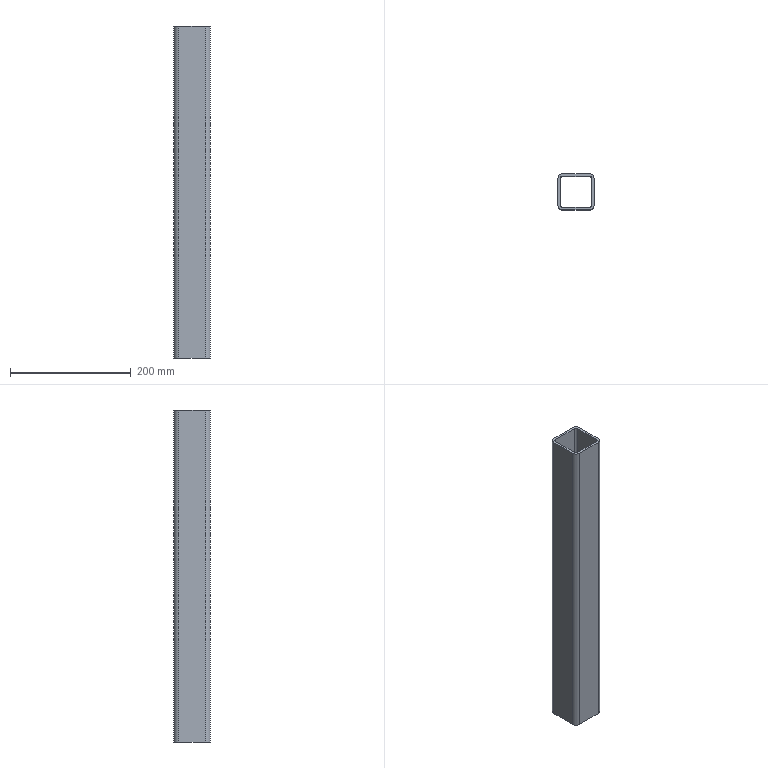Part | SolidWorks | features BaseBody 1 | 1 solid | 18 faces | box 60 x 60 x 550 mm | volume 470138 mm3 | plane 10 | cylinder 8 | commonest cylinder face diameters 8 x4 16 x4
STEP:
#1=CARTESIAN_POINT('',(644.,44.,-1270.));
#2=VERTEX_POINT('',#1);
#3=CARTESIAN_POINT('',(644.,44.,-720.));
#4=VERTEX_POINT('',#3);
#5=CARTESIAN_POINT('',(644.,44.,530.));
#6=DIRECTION('',(0.,0.,1.));
#7=VECTOR('',#6,1000.);
#8=LINE('',#5,#7);
#9=EDGE_CURVE('',#2,#4,#8,.T.);
#10=ORIENTED_EDGE('',*,*,#9,.T.);
#11=CARTESIAN_POINT('',(644.,0.,-720.));
#12=VERTEX_POINT('',#11);
#13=CARTESIAN_POINT('',(644.,44.,-720.));
#14=DIRECTION('',(0.,-1.,0.));
#15=VECTOR('',#14,1000.);
#16=LINE('',#13,#15);
#17=EDGE_CURVE('',#4,#12,#16,.T.);
#18=ORIENTED_EDGE('',*,*,#17,.T.);
#19=CARTESIAN_POINT('',(644.,0.,-1270.));
#20=VERTEX_POINT('',#19);
#21=CARTESIAN_POINT('',(644.,0.,530.));
#22=DIRECTION('',(0.,0.,-1.));
#23=VECTOR('',#22,1000.);
#24=LINE('',#21,#23);
#25=EDGE_CURVE('',#12,#20,#24,.T.);
#26=ORIENTED_EDGE('',*,*,#25,.T.);
#27=CARTESIAN_POINT('',(644.,44.,-1270.));
#28=DIRECTION('',(0.,1.,0.));
#29=VECTOR('',#28,1000.);
#30=LINE('',#27,#29);
#31=EDGE_CURVE('',#20,#2,#30,.T.);
#32=ORIENTED_EDGE('',*,*,#31,.T.);
#33=EDGE_LOOP('',(#10,#18,#26,#32));
#34=FACE_OUTER_BOUND('',#33,.T.);
#35=CARTESIAN_POINT('',(644.,44.,530.));
#36=DIRECTION('',(1.,0.,0.));
#37=DIRECTION('',(0.,0.,-1.));
#38=AXIS2_PLACEMENT_3D('',#35,#36,#37);
#39=PLANE('',#38);
#40=ADVANCED_FACE('',(#34),#39,.T.);
#41=ORIENTED_EDGE('',*,*,#17,.F.);
#42=CARTESIAN_POINT('',(648.,48.,-720.));
#43=VERTEX_POINT('',#42);
#44=CARTESIAN_POINT('',(648.,44.,-720.));
#45=DIRECTION('',(0.,0.,1.));
#46=DIRECTION('',(-1.,0.,0.));
#47=AXIS2_PLACEMENT_3D('',#44,#45,#46);
#48=CIRCLE('',#47,4.);
#49=EDGE_CURVE('',#43,#4,#48,.T.);
#50=ORIENTED_EDGE('',*,*,#49,.F.);
#51=CARTESIAN_POINT('',(692.,48.,-720.));
#52=VERTEX_POINT('',#51);
#53=CARTESIAN_POINT('',(0.,48.,-720.));
#54=DIRECTION('',(-1.,0.,0.));
#55=VECTOR('',#54,1000.);
#56=LINE('',#53,#55);
#57=EDGE_CURVE('',#52,#43,#56,.T.);
#58=ORIENTED_EDGE('',*,*,#57,.F.);
#59=CARTESIAN_POINT('',(696.,44.,-720.));
#60=VERTEX_POINT('',#59);
#61=CARTESIAN_POINT('',(692.,44.,-720.));
#62=DIRECTION('',(0.,0.,1.));
#63=DIRECTION('',(-1.,0.,0.));
#64=AXIS2_PLACEMENT_3D('',#61,#62,#63);
#65=CIRCLE('',#64,4.);
#66=EDGE_CURVE('',#60,#52,#65,.T.);
#67=ORIENTED_EDGE('',*,*,#66,.F.);
#68=CARTESIAN_POINT('',(696.,0.,-720.));
#69=VERTEX_POINT('',#68);
#70=CARTESIAN_POINT('',(696.,1242.,-720.));
#71=DIRECTION('',(0.,1.,0.));
#72=VECTOR('',#71,1000.);
#73=LINE('',#70,#72);
#74=EDGE_CURVE('',#69,#60,#73,.T.);
#75=ORIENTED_EDGE('',*,*,#74,.F.);
#76=CARTESIAN_POINT('',(692.,-4.,-720.));
#77=VERTEX_POINT('',#76);
#78=CARTESIAN_POINT('',(692.,0.,-720.));
#79=DIRECTION('',(0.,0.,1.));
#80=DIRECTION('',(-1.,0.,0.));
#81=AXIS2_PLACEMENT_3D('',#78,#79,#80);
#82=CIRCLE('',#81,4.);
#83=EDGE_CURVE('',#77,#69,#82,.T.);
#84=ORIENTED_EDGE('',*,*,#83,.F.);
#85=CARTESIAN_POINT('',(648.,-4.,-720.));
#86=VERTEX_POINT('',#85);
#87=CARTESIAN_POINT('',(0.,-4.,-720.));
#88=DIRECTION('',(1.,0.,0.));
#89=VECTOR('',#88,1000.);
#90=LINE('',#87,#89);
#91=EDGE_CURVE('',#86,#77,#90,.T.);
#92=ORIENTED_EDGE('',*,*,#91,.F.);
#93=CARTESIAN_POINT('',(648.,0.,-720.));
#94=DIRECTION('',(0.,0.,1.));
#95=DIRECTION('',(-1.,0.,0.));
#96=AXIS2_PLACEMENT_3D('',#93,#94,#95);
#97=CIRCLE('',#96,4.);
#98=EDGE_CURVE('',#12,#86,#97,.T.);
#99=ORIENTED_EDGE('',*,*,#98,.F.);
#100=EDGE_LOOP('',(#41,#50,#58,#67,#75,#84,#92,#99));
#101=FACE_BOUND('',#100,.T.);
#102=CARTESIAN_POINT('',(648.,-8.,-720.));
#103=VERTEX_POINT('',#102);
#104=CARTESIAN_POINT('',(640.,0.,-720.));
#105=VERTEX_POINT('',#104);
#106=CARTESIAN_POINT('',(648.,0.,-720.));
#107=DIRECTION('',(0.,0.,-1.));
#108=DIRECTION('',(-1.,0.,0.));
#109=AXIS2_PLACEMENT_3D('',#106,#107,#108);
#110=CIRCLE('',#109,8.);
#111=EDGE_CURVE('',#103,#105,#110,.T.);
#112=ORIENTED_EDGE('',*,*,#111,.F.);
#113=CARTESIAN_POINT('',(692.,-8.,-720.));
#114=VERTEX_POINT('',#113);
#115=CARTESIAN_POINT('',(0.,-8.,-720.));
#116=DIRECTION('',(-1.,0.,0.));
#117=VECTOR('',#116,1000.);
#118=LINE('',#115,#117);
#119=EDGE_CURVE('',#114,#103,#118,.T.);
#120=ORIENTED_EDGE('',*,*,#119,.F.);
#121=CARTESIAN_POINT('',(700.,0.,-720.));
#122=VERTEX_POINT('',#121);
#123=CARTESIAN_POINT('',(692.,0.,-720.));
#124=DIRECTION('',(0.,0.,-1.));
#125=DIRECTION('',(-1.,0.,0.));
#126=AXIS2_PLACEMENT_3D('',#123,#124,#125);
#127=CIRCLE('',#126,8.);
#128=EDGE_CURVE('',#122,#114,#127,.T.);
#129=ORIENTED_EDGE('',*,*,#128,.F.);
#130=CARTESIAN_POINT('',(700.,44.,-720.));
#131=VERTEX_POINT('',#130);
#132=CARTESIAN_POINT('',(700.,1242.,-720.));
#133=DIRECTION('',(0.,-1.,0.));
#134=VECTOR('',#133,1000.);
#135=LINE('',#132,#134);
#136=EDGE_CURVE('',#131,#122,#135,.T.);
#137=ORIENTED_EDGE('',*,*,#136,.F.);
#138=CARTESIAN_POINT('',(692.,52.,-720.));
#139=VERTEX_POINT('',#138);
#140=CARTESIAN_POINT('',(692.,44.,-720.));
#141=DIRECTION('',(0.,0.,-1.));
#142=DIRECTION('',(-1.,0.,0.));
#143=AXIS2_PLACEMENT_3D('',#140,#141,#142);
#144=CIRCLE('',#143,8.);
#145=EDGE_CURVE('',#139,#131,#144,.T.);
#146=ORIENTED_EDGE('',*,*,#145,.F.);
#147=CARTESIAN_POINT('',(648.,52.,-720.));
#148=VERTEX_POINT('',#147);
#149=CARTESIAN_POINT('',(0.,52.,-720.));
#150=DIRECTION('',(1.,0.,0.));
#151=VECTOR('',#150,1000.);
#152=LINE('',#149,#151);
#153=EDGE_CURVE('',#148,#139,#152,.T.);
#154=ORIENTED_EDGE('',*,*,#153,.F.);
#155=CARTESIAN_POINT('',(640.,44.,-720.));
#156=VERTEX_POINT('',#155);
#157=CARTESIAN_POINT('',(648.,44.,-720.));
#158=DIRECTION('',(0.,0.,-1.));
#159=DIRECTION('',(-1.,0.,0.));
#160=AXIS2_PLACEMENT_3D('',#157,#158,#159);
#161=CIRCLE('',#160,8.);
#162=EDGE_CURVE('',#156,#148,#161,.T.);
#163=ORIENTED_EDGE('',*,*,#162,.F.);
#164=CARTESIAN_POINT('',(640.,1242.,-720.));
#165=DIRECTION('',(0.,1.,0.));
#166=VECTOR('',#165,1000.);
#167=LINE('',#164,#166);
#168=EDGE_CURVE('',#105,#156,#167,.T.);
#169=ORIENTED_EDGE('',*,*,#168,.F.);
#170=EDGE_LOOP('',(#112,#120,#129,#137,#146,#154,#163,#169));
#171=FACE_OUTER_BOUND('',#170,.T.);
#172=CARTESIAN_POINT('',(0.,1242.,-720.));
#173=DIRECTION('',(0.,0.,-1.));
#174=DIRECTION('',(-1.,0.,0.));
#175=AXIS2_PLACEMENT_3D('',#172,#173,#174);
#176=PLANE('',#175);
#177=ADVANCED_FACE('',(#101,#171),#176,.F.);
#178=CARTESIAN_POINT('',(648.,48.,-1270.));
#179=VERTEX_POINT('',#178);
#180=CARTESIAN_POINT('',(648.,44.,-1270.));
#181=DIRECTION('',(0.,0.,1.));
#182=DIRECTION('',(-1.,0.,0.));
#183=AXIS2_PLACEMENT_3D('',#180,#181,#182);
#184=CIRCLE('',#183,4.);
#185=EDGE_CURVE('',#179,#2,#184,.T.);
#186=ORIENTED_EDGE('',*,*,#185,.F.);
#187=CARTESIAN_POINT('',(648.,48.,530.));
#188=DIRECTION('',(0.,0.,-1.));
#189=VECTOR('',#188,1000.);
#190=LINE('',#187,#189);
#191=EDGE_CURVE('',#43,#179,#190,.T.);
#192=ORIENTED_EDGE('',*,*,#191,.F.);
#193=ORIENTED_EDGE('',*,*,#49,.T.);
#194=ORIENTED_EDGE('',*,*,#9,.F.);
#195=EDGE_LOOP('',(#186,#192,#193,#194));
#196=FACE_OUTER_BOUND('',#195,.T.);
#197=CARTESIAN_POINT('',(648.,44.,530.));
#198=DIRECTION('',(0.,0.,-1.));
#199=DIRECTION('',(-1.,0.,0.));
#200=AXIS2_PLACEMENT_3D('',#197,#198,#199);
#201=CYLINDRICAL_SURFACE('',#200,4.);
#202=ADVANCED_FACE('',(#196),#201,.F.);
#203=CARTESIAN_POINT('',(696.,0.,-1270.));
#204=VERTEX_POINT('',#203);
#205=CARTESIAN_POINT('',(692.,-4.,-1270.));
#206=VERTEX_POINT('',#205);
#207=CARTESIAN_POINT('',(692.,0.,-1270.));
#208=DIRECTION('',(0.,0.,-1.));
#209=DIRECTION('',(-1.,0.,0.));
#210=AXIS2_PLACEMENT_3D('',#207,#208,#209);
#211=CIRCLE('',#210,4.);
#212=EDGE_CURVE('',#204,#206,#211,.T.);
#213=ORIENTED_EDGE('',*,*,#212,.F.);
#214=CARTESIAN_POINT('',(696.,44.,-1270.));
#215=VERTEX_POINT('',#214);
#216=CARTESIAN_POINT('',(696.,44.,-1270.));
#217=DIRECTION('',(0.,-1.,0.));
#218=VECTOR('',#217,1000.);
#219=LINE('',#216,#218);
#220=EDGE_CURVE('',#215,#204,#219,.T.);
#221=ORIENTED_EDGE('',*,*,#220,.F.);
#222=CARTESIAN_POINT('',(692.,48.,-1270.));
#223=VERTEX_POINT('',#222);
#224=CARTESIAN_POINT('',(692.,44.,-1270.));
#225=DIRECTION('',(0.,0.,-1.));
#226=DIRECTION('',(-1.,0.,0.));
#227=AXIS2_PLACEMENT_3D('',#224,#225,#226);
#228=CIRCLE('',#227,4.);
#229=EDGE_CURVE('',#223,#215,#228,.T.);
#230=ORIENTED_EDGE('',*,*,#229,.F.);
#231=CARTESIAN_POINT('',(648.,48.,-1270.));
#232=DIRECTION('',(1.,0.,0.));
#233=VECTOR('',#232,1000.);
#234=LINE('',#231,#233);
#235=EDGE_CURVE('',#179,#223,#234,.T.);
#236=ORIENTED_EDGE('',*,*,#235,.F.);
#237=ORIENTED_EDGE('',*,*,#185,.T.);
#238=ORIENTED_EDGE('',*,*,#31,.F.);
#239=CARTESIAN_POINT('',(648.,-4.,-1270.));
#240=VERTEX_POINT('',#239);
#241=CARTESIAN_POINT('',(648.,0.,-1270.));
#242=DIRECTION('',(0.,0.,-1.));
#243=DIRECTION('',(-1.,0.,0.));
#244=AXIS2_PLACEMENT_3D('',#241,#242,#243);
#245=CIRCLE('',#244,4.);
#246=EDGE_CURVE('',#240,#20,#245,.T.);
#247=ORIENTED_EDGE('',*,*,#246,.F.);
#248=CARTESIAN_POINT('',(648.,-4.,-1270.));
#249=DIRECTION('',(-1.,0.,0.));
#250=VECTOR('',#249,1000.);
#251=LINE('',#248,#250);
#252=EDGE_CURVE('',#206,#240,#251,.T.);
#253=ORIENTED_EDGE('',*,*,#252,.F.);
#254=EDGE_LOOP('',(#213,#221,#230,#236,#237,#238,#247,#253));
#255=FACE_BOUND('',#254,.T.);
#256=CARTESIAN_POINT('',(700.,44.,-1270.));
#257=VERTEX_POINT('',#256);
#258=CARTESIAN_POINT('',(692.,52.,-1270.));
#259=VERTEX_POINT('',#258);
#260=CARTESIAN_POINT('',(692.,44.,-1270.));
#261=DIRECTION('',(0.,0.,1.));
#262=DIRECTION('',(-1.,0.,0.));
#263=AXIS2_PLACEMENT_3D('',#260,#261,#262);
#264=CIRCLE('',#263,8.);
#265=EDGE_CURVE('',#257,#259,#264,.T.);
#266=ORIENTED_EDGE('',*,*,#265,.F.);
#267=CARTESIAN_POINT('',(700.,0.,-1270.));
#268=VERTEX_POINT('',#267);
#269=CARTESIAN_POINT('',(700.,44.,-1270.));
#270=DIRECTION('',(0.,1.,0.));
#271=VECTOR('',#270,1000.);
#272=LINE('',#269,#271);
#273=EDGE_CURVE('',#268,#257,#272,.T.);
#274=ORIENTED_EDGE('',*,*,#273,.F.);
#275=CARTESIAN_POINT('',(692.,-8.,-1270.));
#276=VERTEX_POINT('',#275);
#277=CARTESIAN_POINT('',(692.,0.,-1270.));
#278=DIRECTION('',(0.,0.,1.));
#279=DIRECTION('',(-1.,0.,0.));
#280=AXIS2_PLACEMENT_3D('',#277,#278,#279);
#281=CIRCLE('',#280,8.);
#282=EDGE_CURVE('',#276,#268,#281,.T.);
#283=ORIENTED_EDGE('',*,*,#282,.F.);
#284=CARTESIAN_POINT('',(648.,-8.,-1270.));
#285=VERTEX_POINT('',#284);
#286=CARTESIAN_POINT('',(648.,-8.,-1270.));
#287=DIRECTION('',(1.,0.,0.));
#288=VECTOR('',#287,1000.);
#289=LINE('',#286,#288);
#290=EDGE_CURVE('',#285,#276,#289,.T.);
#291=ORIENTED_EDGE('',*,*,#290,.F.);
#292=CARTESIAN_POINT('',(640.,0.,-1270.));
#293=VERTEX_POINT('',#292);
#294=CARTESIAN_POINT('',(648.,0.,-1270.));
#295=DIRECTION('',(0.,0.,1.));
#296=DIRECTION('',(-1.,0.,0.));
#297=AXIS2_PLACEMENT_3D('',#294,#295,#296);
#298=CIRCLE('',#297,8.);
#299=EDGE_CURVE('',#293,#285,#298,.T.);
#300=ORIENTED_EDGE('',*,*,#299,.F.);
#301=CARTESIAN_POINT('',(640.,44.,-1270.));
#302=VERTEX_POINT('',#301);
#303=CARTESIAN_POINT('',(640.,44.,-1270.));
#304=DIRECTION('',(0.,-1.,0.));
#305=VECTOR('',#304,1000.);
#306=LINE('',#303,#305);
#307=EDGE_CURVE('',#302,#293,#306,.T.);
#308=ORIENTED_EDGE('',*,*,#307,.F.);
#309=CARTESIAN_POINT('',(648.,52.,-1270.));
#310=VERTEX_POINT('',#309);
#311=CARTESIAN_POINT('',(648.,44.,-1270.));
#312=DIRECTION('',(0.,0.,1.));
#313=DIRECTION('',(-1.,0.,0.));
#314=AXIS2_PLACEMENT_3D('',#311,#312,#313);
#315=CIRCLE('',#314,8.);
#316=EDGE_CURVE('',#310,#302,#315,.T.);
#317=ORIENTED_EDGE('',*,*,#316,.F.);
#318=CARTESIAN_POINT('',(648.,52.,-1270.));
#319=DIRECTION('',(-1.,0.,0.));
#320=VECTOR('',#319,1000.);
#321=LINE('',#318,#320);
#322=EDGE_CURVE('',#259,#310,#321,.T.);
#323=ORIENTED_EDGE('',*,*,#322,.F.);
#324=EDGE_LOOP('',(#266,#274,#283,#291,#300,#308,#317,#323));
#325=FACE_OUTER_BOUND('',#324,.T.);
#326=CARTESIAN_POINT('',(648.,44.,-1270.));
#327=DIRECTION('',(0.,0.,1.));
#328=DIRECTION('',(1.,0.,0.));
#329=AXIS2_PLACEMENT_3D('',#326,#327,#328);
#330=PLANE('',#329);
#331=ADVANCED_FACE('',(#255,#325),#330,.F.);
#332=ORIENTED_EDGE('',*,*,#246,.T.);
#333=ORIENTED_EDGE('',*,*,#25,.F.);
#334=ORIENTED_EDGE('',*,*,#98,.T.);
#335=CARTESIAN_POINT('',(648.,-4.,530.));
#336=DIRECTION('',(0.,0.,1.));
#337=VECTOR('',#336,1000.);
#338=LINE('',#335,#337);
#339=EDGE_CURVE('',#240,#86,#338,.T.);
#340=ORIENTED_EDGE('',*,*,#339,.F.);
#341=EDGE_LOOP('',(#332,#333,#334,#340));
#342=FACE_OUTER_BOUND('',#341,.T.);
#343=CARTESIAN_POINT('',(648.,0.,530.));
#344=DIRECTION('',(0.,0.,-1.));
#345=DIRECTION('',(-1.,0.,0.));
#346=AXIS2_PLACEMENT_3D('',#343,#344,#345);
#347=CYLINDRICAL_SURFACE('',#346,4.);
#348=ADVANCED_FACE('',(#342),#347,.F.);
#349=CARTESIAN_POINT('',(692.,48.,530.));
#350=DIRECTION('',(0.,0.,1.));
#351=VECTOR('',#350,1000.);
#352=LINE('',#349,#351);
#353=EDGE_CURVE('',#223,#52,#352,.T.);
#354=ORIENTED_EDGE('',*,*,#353,.T.);
#355=ORIENTED_EDGE('',*,*,#57,.T.);
#356=ORIENTED_EDGE('',*,*,#191,.T.);
#357=ORIENTED_EDGE('',*,*,#235,.T.);
#358=EDGE_LOOP('',(#354,#355,#356,#357));
#359=FACE_OUTER_BOUND('',#358,.T.);
#360=CARTESIAN_POINT('',(648.,48.,530.));
#361=DIRECTION('',(0.,-1.,0.));
#362=DIRECTION('',(0.,0.,-1.));
#363=AXIS2_PLACEMENT_3D('',#360,#361,#362);
#364=PLANE('',#363);
#365=ADVANCED_FACE('',(#359),#364,.T.);
#366=ORIENTED_EDGE('',*,*,#229,.T.);
#367=CARTESIAN_POINT('',(696.,44.,530.));
#368=DIRECTION('',(0.,0.,-1.));
#369=VECTOR('',#368,1000.);
#370=LINE('',#367,#369);
#371=EDGE_CURVE('',#60,#215,#370,.T.);
#372=ORIENTED_EDGE('',*,*,#371,.F.);
#373=ORIENTED_EDGE('',*,*,#66,.T.);
#374=ORIENTED_EDGE('',*,*,#353,.F.);
#375=EDGE_LOOP('',(#366,#372,#373,#374));
#376=FACE_OUTER_BOUND('',#375,.T.);
#377=CARTESIAN_POINT('',(692.,44.,530.));
#378=DIRECTION('',(0.,0.,-1.));
#379=DIRECTION('',(-1.,0.,0.));
#380=AXIS2_PLACEMENT_3D('',#377,#378,#379);
#381=CYLINDRICAL_SURFACE('',#380,4.);
#382=ADVANCED_FACE('',(#376),#381,.F.);
#383=CARTESIAN_POINT('',(696.,0.,530.));
#384=DIRECTION('',(0.,0.,1.));
#385=VECTOR('',#384,1000.);
#386=LINE('',#383,#385);
#387=EDGE_CURVE('',#204,#69,#386,.T.);
#388=ORIENTED_EDGE('',*,*,#387,.T.);
#389=ORIENTED_EDGE('',*,*,#74,.T.);
#390=ORIENTED_EDGE('',*,*,#371,.T.);
#391=ORIENTED_EDGE('',*,*,#220,.T.);
#392=EDGE_LOOP('',(#388,#389,#390,#391));
#393=FACE_OUTER_BOUND('',#392,.T.);
#394=CARTESIAN_POINT('',(696.,0.,530.));
#395=DIRECTION('',(-1.,0.,0.));
#396=DIRECTION('',(0.,0.,1.));
#397=AXIS2_PLACEMENT_3D('',#394,#395,#396);
#398=PLANE('',#397);
#399=ADVANCED_FACE('',(#393),#398,.T.);
#400=ORIENTED_EDGE('',*,*,#212,.T.);
#401=CARTESIAN_POINT('',(692.,-4.,530.));
#402=DIRECTION('',(0.,0.,-1.));
#403=VECTOR('',#402,1000.);
#404=LINE('',#401,#403);
#405=EDGE_CURVE('',#77,#206,#404,.T.);
#406=ORIENTED_EDGE('',*,*,#405,.F.);
#407=ORIENTED_EDGE('',*,*,#83,.T.);
#408=ORIENTED_EDGE('',*,*,#387,.F.);
#409=EDGE_LOOP('',(#400,#406,#407,#408));
#410=FACE_OUTER_BOUND('',#409,.T.);
#411=CARTESIAN_POINT('',(692.,0.,530.));
#412=DIRECTION('',(0.,0.,-1.));
#413=DIRECTION('',(-1.,0.,0.));
#414=AXIS2_PLACEMENT_3D('',#411,#412,#413);
#415=CYLINDRICAL_SURFACE('',#414,4.);
#416=ADVANCED_FACE('',(#410),#415,.F.);
#417=ORIENTED_EDGE('',*,*,#339,.T.);
#418=ORIENTED_EDGE('',*,*,#91,.T.);
#419=ORIENTED_EDGE('',*,*,#405,.T.);
#420=ORIENTED_EDGE('',*,*,#252,.T.);
#421=EDGE_LOOP('',(#417,#418,#419,#420));
#422=FACE_OUTER_BOUND('',#421,.T.);
#423=CARTESIAN_POINT('',(692.,-4.,530.));
#424=DIRECTION('',(0.,1.,0.));
#425=DIRECTION('',(0.,0.,1.));
#426=AXIS2_PLACEMENT_3D('',#423,#424,#425);
#427=PLANE('',#426);
#428=ADVANCED_FACE('',(#422),#427,.T.);
#429=CARTESIAN_POINT('',(640.,44.,530.));
#430=DIRECTION('',(0.,0.,1.));
#431=VECTOR('',#430,1000.);
#432=LINE('',#429,#431);
#433=EDGE_CURVE('',#302,#156,#432,.T.);
#434=ORIENTED_EDGE('',*,*,#433,.F.);
#435=ORIENTED_EDGE('',*,*,#307,.T.);
#436=CARTESIAN_POINT('',(640.,0.,530.));
#437=DIRECTION('',(0.,0.,-1.));
#438=VECTOR('',#437,1000.);
#439=LINE('',#436,#438);
#440=EDGE_CURVE('',#105,#293,#439,.T.);
#441=ORIENTED_EDGE('',*,*,#440,.F.);
#442=ORIENTED_EDGE('',*,*,#168,.T.);
#443=EDGE_LOOP('',(#434,#435,#441,#442));
#444=FACE_OUTER_BOUND('',#443,.T.);
#445=CARTESIAN_POINT('',(640.,44.,530.));
#446=DIRECTION('',(1.,0.,0.));
#447=DIRECTION('',(0.,0.,-1.));
#448=AXIS2_PLACEMENT_3D('',#445,#446,#447);
#449=PLANE('',#448);
#450=ADVANCED_FACE('',(#444),#449,.F.);
#451=ORIENTED_EDGE('',*,*,#299,.T.);
#452=CARTESIAN_POINT('',(648.,-8.,530.));
#453=DIRECTION('',(0.,0.,1.));
#454=VECTOR('',#453,1000.);
#455=LINE('',#452,#454);
#456=EDGE_CURVE('',#285,#103,#455,.T.);
#457=ORIENTED_EDGE('',*,*,#456,.T.);
#458=ORIENTED_EDGE('',*,*,#111,.T.);
#459=ORIENTED_EDGE('',*,*,#440,.T.);
#460=EDGE_LOOP('',(#451,#457,#458,#459));
#461=FACE_OUTER_BOUND('',#460,.T.);
#462=CARTESIAN_POINT('',(648.,0.,530.));
#463=DIRECTION('',(0.,0.,-1.));
#464=DIRECTION('',(-1.,0.,0.));
#465=AXIS2_PLACEMENT_3D('',#462,#463,#464);
#466=CYLINDRICAL_SURFACE('',#465,8.);
#467=ADVANCED_FACE('',(#461),#466,.T.);
#468=ORIENTED_EDGE('',*,*,#456,.F.);
#469=ORIENTED_EDGE('',*,*,#290,.T.);
#470=CARTESIAN_POINT('',(692.,-8.,530.));
#471=DIRECTION('',(0.,0.,-1.));
#472=VECTOR('',#471,1000.);
#473=LINE('',#470,#472);
#474=EDGE_CURVE('',#114,#276,#473,.T.);
#475=ORIENTED_EDGE('',*,*,#474,.F.);
#476=ORIENTED_EDGE('',*,*,#119,.T.);
#477=EDGE_LOOP('',(#468,#469,#475,#476));
#478=FACE_OUTER_BOUND('',#477,.T.);
#479=CARTESIAN_POINT('',(692.,-8.,530.));
#480=DIRECTION('',(0.,1.,0.));
#481=DIRECTION('',(0.,0.,1.));
#482=AXIS2_PLACEMENT_3D('',#479,#480,#481);
#483=PLANE('',#482);
#484=ADVANCED_FACE('',(#478),#483,.F.);
#485=ORIENTED_EDGE('',*,*,#282,.T.);
#486=CARTESIAN_POINT('',(700.,0.,530.));
#487=DIRECTION('',(0.,0.,1.));
#488=VECTOR('',#487,1000.);
#489=LINE('',#486,#488);
#490=EDGE_CURVE('',#268,#122,#489,.T.);
#491=ORIENTED_EDGE('',*,*,#490,.T.);
#492=ORIENTED_EDGE('',*,*,#128,.T.);
#493=ORIENTED_EDGE('',*,*,#474,.T.);
#494=EDGE_LOOP('',(#485,#491,#492,#493));
#495=FACE_OUTER_BOUND('',#494,.T.);
#496=CARTESIAN_POINT('',(692.,0.,530.));
#497=DIRECTION('',(0.,0.,-1.));
#498=DIRECTION('',(-1.,0.,0.));
#499=AXIS2_PLACEMENT_3D('',#496,#497,#498);
#500=CYLINDRICAL_SURFACE('',#499,8.);
#501=ADVANCED_FACE('',(#495),#500,.T.);
#502=ORIENTED_EDGE('',*,*,#490,.F.);
#503=ORIENTED_EDGE('',*,*,#273,.T.);
#504=CARTESIAN_POINT('',(700.,44.,530.));
#505=DIRECTION('',(0.,0.,-1.));
#506=VECTOR('',#505,1000.);
#507=LINE('',#504,#506);
#508=EDGE_CURVE('',#131,#257,#507,.T.);
#509=ORIENTED_EDGE('',*,*,#508,.F.);
#510=ORIENTED_EDGE('',*,*,#136,.T.);
#511=EDGE_LOOP('',(#502,#503,#509,#510));
#512=FACE_OUTER_BOUND('',#511,.T.);
#513=CARTESIAN_POINT('',(700.,0.,530.));
#514=DIRECTION('',(-1.,0.,0.));
#515=DIRECTION('',(0.,0.,1.));
#516=AXIS2_PLACEMENT_3D('',#513,#514,#515);
#517=PLANE('',#516);
#518=ADVANCED_FACE('',(#512),#517,.F.);
#519=ORIENTED_EDGE('',*,*,#265,.T.);
#520=CARTESIAN_POINT('',(692.,52.,530.));
#521=DIRECTION('',(0.,0.,1.));
#522=VECTOR('',#521,1000.);
#523=LINE('',#520,#522);
#524=EDGE_CURVE('',#259,#139,#523,.T.);
#525=ORIENTED_EDGE('',*,*,#524,.T.);
#526=ORIENTED_EDGE('',*,*,#145,.T.);
#527=ORIENTED_EDGE('',*,*,#508,.T.);
#528=EDGE_LOOP('',(#519,#525,#526,#527));
#529=FACE_OUTER_BOUND('',#528,.T.);
#530=CARTESIAN_POINT('',(692.,44.,530.));
#531=DIRECTION('',(0.,0.,-1.));
#532=DIRECTION('',(-1.,0.,0.));
#533=AXIS2_PLACEMENT_3D('',#530,#531,#532);
#534=CYLINDRICAL_SURFACE('',#533,8.);
#535=ADVANCED_FACE('',(#529),#534,.T.);
#536=ORIENTED_EDGE('',*,*,#524,.F.);
#537=ORIENTED_EDGE('',*,*,#322,.T.);
#538=CARTESIAN_POINT('',(648.,52.,530.));
#539=DIRECTION('',(0.,0.,-1.));
#540=VECTOR('',#539,1000.);
#541=LINE('',#538,#540);
#542=EDGE_CURVE('',#148,#310,#541,.T.);
#543=ORIENTED_EDGE('',*,*,#542,.F.);
#544=ORIENTED_EDGE('',*,*,#153,.T.);
#545=EDGE_LOOP('',(#536,#537,#543,#544));
#546=FACE_OUTER_BOUND('',#545,.T.);
#547=CARTESIAN_POINT('',(648.,52.,530.));
#548=DIRECTION('',(0.,-1.,0.));
#549=DIRECTION('',(0.,0.,-1.));
#550=AXIS2_PLACEMENT_3D('',#547,#548,#549);
#551=PLANE('',#550);
#552=ADVANCED_FACE('',(#546),#551,.F.);
#553=ORIENTED_EDGE('',*,*,#316,.T.);
#554=ORIENTED_EDGE('',*,*,#433,.T.);
#555=ORIENTED_EDGE('',*,*,#162,.T.);
#556=ORIENTED_EDGE('',*,*,#542,.T.);
#557=EDGE_LOOP('',(#553,#554,#555,#556));
#558=FACE_OUTER_BOUND('',#557,.T.);
#559=CARTESIAN_POINT('',(648.,44.,530.));
#560=DIRECTION('',(0.,0.,-1.));
#561=DIRECTION('',(-1.,0.,0.));
#562=AXIS2_PLACEMENT_3D('',#559,#560,#561);
#563=CYLINDRICAL_SURFACE('',#562,8.);
#564=ADVANCED_FACE('',(#558),#563,.T.);
#565=CLOSED_SHELL('',(#40,#177,#202,#331,#348,#365,#382,#399,#416,#428,#450,#467,#484,#501,#518,#535,#552,#564));
#566=MANIFOLD_SOLID_BREP('',#565);
#567=CARTESIAN_POINT('',(0.,0.,0.));
#568=DIRECTION('',(0.,0.,1.));
#569=DIRECTION('',(1.,0.,0.));
#570=AXIS2_PLACEMENT_3D('',#567,#568,#569);
#571=(LENGTH_UNIT()NAMED_UNIT(*)SI_UNIT(.MILLI.,.METRE.));
#572=UNCERTAINTY_MEASURE_WITH_UNIT(LENGTH_MEASURE(0.00001),#571,'','');
#573=(NAMED_UNIT(*)PLANE_ANGLE_UNIT()SI_UNIT($,.RADIAN.));
#574=(NAMED_UNIT(*)SI_UNIT($,.STERADIAN.)SOLID_ANGLE_UNIT());
#575=(GEOMETRIC_REPRESENTATION_CONTEXT(3)GLOBAL_UNCERTAINTY_ASSIGNED_CONTEXT((#572))GLOBAL_UNIT_ASSIGNED_CONTEXT((#571,#573,#574))REPRESENTATION_CONTEXT('',''));
#576=ADVANCED_BREP_SHAPE_REPRESENTATION('',(#566,#570),#575);